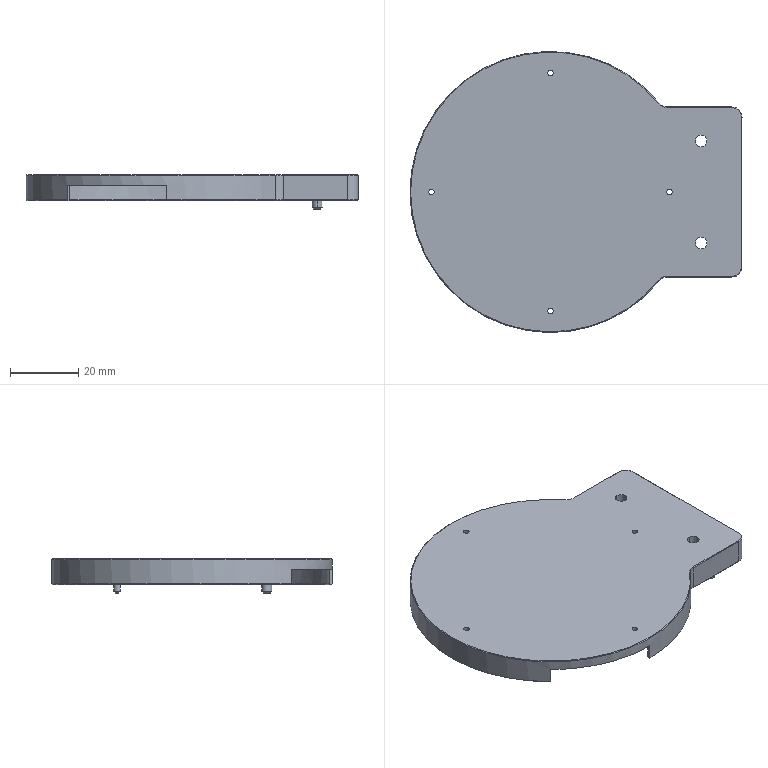NC program | NX | posted with a generic post | part box 97.6 x 82.6 x 10 mm
Lines 2561 to 3495 of 4898:
(CAVITY_MILL_COPY_COPY , TOOL : D3)
N5108 T17 M6
N5110 G54
N5112 G17 G0 G90 X20.005 Y-45.7 S9500 M3
N5114 G43 Z30. H17
N5116 Z-2.196
N5118 G94 G1 Z-2.696 F1000.
N5120 X20.062 Y-45.8
N5122 G3 X20.928 Y-46.3 R1.
N5124 G1 X21.5 F1100.
N5126 G3 X22.5 Y-45.3 R1.
N5128 G1 Y-44.728
N5130 G3 X22. Y-43.862 R1.
N5132 G1 X21.9 Y-43.805
N5134 Z-2.196
N5136 G0 X20.005 Y-45.7 Z-2.391
N5138 G1 Z-2.891 F1000.
N5140 X20.062 Y-45.8
N5142 G3 X20.928 Y-46.3 R1.
N5144 G1 X21.5 F1100.
N5146 G3 X22.5 Y-45.3 R1.
N5148 G1 Y-44.728
N5150 G3 X22. Y-43.862 R1.
N5152 G1 X21.9 Y-43.805
N5154 Z-2.391
N5156 G0 X20.005 Y-45.7 Z-2.587
N5158 G1 Z-3.087 F1000.
N5160 X20.062 Y-45.8
N5162 G3 X20.928 Y-46.3 R1.
N5164 G1 X21.5 F1100.
N5166 G3 X22.5 Y-45.3 R1.
N5168 G1 Y-44.728
N5170 G3 X22. Y-43.862 R1.
N5172 G1 X21.9 Y-43.805
N5174 Z-2.587
N5176 G0 X20.005 Y-45.7 Z-2.783
N5178 G1 Z-3.283 F1000.
N5180 X20.062 Y-45.8
N5182 G3 X20.928 Y-46.3 R1.
N5184 G1 X21.5 F1100.
N5186 G3 X22.5 Y-45.3 R1.
N5188 G1 Y-44.728
N5190 G3 X22. Y-43.862 R1.
N5192 G1 X21.9 Y-43.805
N5194 Z-2.783
N5196 G0 X20.005 Y-45.7 Z-2.978
N5198 G1 Z-3.478 F1000.
N5200 X20.062 Y-45.8
N5202 G3 X20.928 Y-46.3 R1.
N5204 G1 X21.5 F1100.
N5206 G3 X22.5 Y-45.3 R1.
N5208 G1 Y-44.728
N5210 G3 X22. Y-43.862 R1.
N5212 G1 X21.9 Y-43.805
N5214 Z-2.978
N5216 G0 X20.005 Y-45.7 Z-3.174
N5218 G1 Z-3.674 F1000.
N5220 X20.062 Y-45.8
N5222 G3 X20.928 Y-46.3 R1.
N5224 G1 X21.5 F1100.
N5226 G3 X22.5 Y-45.3 R1.
N5228 G1 Y-44.728
N5230 G3 X22. Y-43.862 R1.
N5232 G1 X21.9 Y-43.805
N5234 Z-3.174
N5236 G0 X20.005 Y-45.7 Z-3.37
N5238 G1 Z-3.87 F1000.
N5240 X20.062 Y-45.8
N5242 G3 X20.928 Y-46.3 R1.
N5244 G1 X21.5 F1100.
N5246 G3 X22.5 Y-45.3 R1.
N5248 G1 Y-44.728
N5250 G3 X22. Y-43.862 R1.
N5252 G1 X21.9 Y-43.805
N5254 Z-3.37
N5256 G0 X20.005 Y-45.7 Z-3.565
N5258 G1 Z-4.065 F1000.
N5260 X20.062 Y-45.8
N5262 G3 X20.928 Y-46.3 R1.
N5264 G1 X21.5 F1100.
N5266 G3 X22.5 Y-45.3 R1.
N5268 G1 Y-44.728
N5270 G3 X22. Y-43.862 R1.
N5272 G1 X21.9 Y-43.805
N5274 Z-3.565
N5276 G0 X20.005 Y-45.7 Z-3.761
N5278 G1 Z-4.261 F1000.
N5280 X20.062 Y-45.8
N5282 G3 X20.928 Y-46.3 R1.
N5284 G1 X21.5 F1100.
N5286 G3 X22.5 Y-45.3 R1.
N5288 G1 Y-44.728
N5290 G3 X22. Y-43.862 R1.
N5292 G1 X21.9 Y-43.805
N5294 Z-3.761
N5296 G0 X20.005 Y-45.7 Z-3.957
N5298 G1 Z-4.457 F1000.
N5300 X20.062 Y-45.8
N5302 G3 X20.928 Y-46.3 R1.
N5304 G1 X21.5 F1100.
N5306 G3 X22.5 Y-45.3 R1.
N5308 G1 Y-44.728
N5310 G3 X22. Y-43.862 R1.
N5312 G1 X21.9 Y-43.805
N5314 Z-3.957
N5316 G0 X20.005 Y-45.7 Z-4.152
N5318 G1 Z-4.652 F1000.
N5320 X20.062 Y-45.8
N5322 G3 X20.928 Y-46.3 R1.
N5324 G1 X21.5 F1100.
N5326 G3 X22.5 Y-45.3 R1.
N5328 G1 Y-44.728
N5330 G3 X22. Y-43.862 R1.
N5332 G1 X21.9 Y-43.805
N5334 Z-4.152
N5336 G0 X20.005 Y-45.7 Z-4.348
N5338 G1 Z-4.848 F1000.
N5340 X20.062 Y-45.8
N5342 G3 X20.928 Y-46.3 R1.
N5344 G1 X21.5 F1100.
N5346 G3 X22.5 Y-45.3 R1.
N5348 G1 Y-44.728
N5350 G3 X22. Y-43.862 R1.
N5352 G1 X21.9 Y-43.805
N5354 Z-4.348
N5356 G0 X20.005 Y-45.7 Z-4.543
N5358 G1 Z-5.043 F1000.
N5360 X20.062 Y-45.8
N5362 G3 X20.928 Y-46.3 R1.
N5364 G1 X21.5 F1100.
N5366 G3 X22.5 Y-45.3 R1.
N5368 G1 Y-44.728
N5370 G3 X22. Y-43.862 R1.
N5372 G1 X21.9 Y-43.805
N5374 Z-4.543
N5376 G0 X20.005 Y-45.7 Z-4.739
N5378 G1 Z-5.239 F1000.
N5380 X20.062 Y-45.8
N5382 G3 X20.928 Y-46.3 R1.
N5384 G1 X21.5 F1100.
N5386 G3 X22.5 Y-45.3 R1.
N5388 G1 Y-44.728
N5390 G3 X22. Y-43.862 R1.
N5392 G1 X21.9 Y-43.805
N5394 Z-4.739
N5396 G0 X20.005 Y-45.7 Z-4.935
N5398 G1 Z-5.435 F1000.
N5400 X20.062 Y-45.8
N5402 G3 X20.928 Y-46.3 R1.
N5404 G1 X21.5 F1100.
N5406 G3 X22.5 Y-45.3 R1.
N5408 G1 Y-44.728
N5410 G3 X22. Y-43.862 R1.
N5412 G1 X21.9 Y-43.805
N5414 Z-4.935
N5416 G0 X20.005 Y-45.7 Z-5.13
N5418 G1 Z-5.63 F1000.
N5420 X20.062 Y-45.8
N5422 G3 X20.928 Y-46.3 R1.
N5424 G1 X21.5 F1100.
N5426 G3 X22.5 Y-45.3 R1.
N5428 G1 Y-44.728
N5430 G3 X22. Y-43.862 R1.
N5432 G1 X21.9 Y-43.805
N5434 Z-5.13
N5436 G0 X20.005 Y-45.7 Z-5.326
N5438 G1 Z-5.826 F1000.
N5440 X20.062 Y-45.8
N5442 G3 X20.928 Y-46.3 R1.
N5444 G1 X21.5 F1100.
N5446 G3 X22.5 Y-45.3 R1.
N5448 G1 Y-44.728
N5450 G3 X22. Y-43.862 R1.
N5452 G1 X21.9 Y-43.805
N5454 Z-5.326
N5456 G0 X20.005 Y-45.7 Z-5.522
N5458 G1 Z-6.022 F1000.
N5460 X20.062 Y-45.8
N5462 G3 X20.928 Y-46.3 R1.
N5464 G1 X21.5 F1100.
N5466 G3 X22.5 Y-45.3 R1.
N5468 G1 Y-44.728
N5470 G3 X22. Y-43.862 R1.
N5472 G1 X21.9 Y-43.805
N5474 Z-5.522
N5476 G0 X20.005 Y-45.7 Z-5.717
N5478 G1 Z-6.217 F1000.
N5480 X20.062 Y-45.8
N5482 G3 X20.928 Y-46.3 R1.
N5484 G1 X21.5 F1100.
N5486 G3 X22.5 Y-45.3 R1.
N5488 G1 Y-44.728
N5490 G3 X22. Y-43.862 R1.
N5492 G1 X21.9 Y-43.805
N5494 Z-5.717
N5496 G0 X20.005 Y-45.7 Z-5.913
N5498 G1 Z-6.413 F1000.
N5500 X20.062 Y-45.8
N5502 G3 X20.928 Y-46.3 R1.
N5504 G1 X21.5 F1100.
N5506 G3 X22.5 Y-45.3 R1.
N5508 G1 Y-44.728
N5510 G3 X22. Y-43.862 R1.
N5512 G1 X21.9 Y-43.805
N5514 Z-5.913
N5516 G0 X20.005 Y-45.7 Z-6.109
N5518 G1 Z-6.609 F1000.
N5520 X20.062 Y-45.8
N5522 G3 X20.928 Y-46.3 R1.
N5524 G1 X21.5 F1100.
N5526 G3 X22.5 Y-45.3 R1.
N5528 G1 Y-44.728
N5530 G3 X22. Y-43.862 R1.
N5532 G1 X21.9 Y-43.805
N5534 Z-6.109
N5536 G0 X20.005 Y-45.7 Z-6.304
N5538 G1 Z-6.804 F1000.
N5540 X20.062 Y-45.8
N5542 G3 X20.928 Y-46.3 R1.
N5544 G1 X21.5 F1100.
N5546 G3 X22.5 Y-45.3 R1.
N5548 G1 Y-44.728
N5550 G3 X22. Y-43.862 R1.
N5552 G1 X21.9 Y-43.805
N5554 Z-6.304
N5556 G0 X20.005 Y-45.7 Z-6.5
N5558 G1 Z-7. F1000.
N5560 X20.062 Y-45.8
N5562 G3 X20.928 Y-46.3 R1.
N5564 G1 X21.5 F1100.
N5566 G3 X22.5 Y-45.3 R1.
N5568 G1 Y-44.728
N5570 G3 X22. Y-43.862 R1.
N5572 G1 X21.9 Y-43.805
N5574 Z-6.5
N5576 G0 X20.005 Y-45.7 Z-6.7
N5578 G1 Z-7.2 F1000.
N5580 X20.062 Y-45.8
N5582 G3 X20.928 Y-46.3 R1.
N5584 G1 X21.5 F1100.
N5586 G3 X22.5 Y-45.3 R1.
N5588 G1 Y-44.728
N5590 G3 X22. Y-43.862 R1.
N5592 G1 X21.9 Y-43.805
N5594 Z-6.7
N5596 G0 X20.005 Y-45.7 Z-6.9
N5598 G1 Z-7.4 F1000.
N5600 X20.062 Y-45.8
N5602 G3 X20.928 Y-46.3 R1.
N5604 G1 X21.5 F1100.
N5606 G3 X22.5 Y-45.3 R1.
N5608 G1 Y-44.728
N5610 G3 X22. Y-43.862 R1.
N5612 G1 X21.9 Y-43.805
N5614 Z-6.9
N5616 G0 X20.005 Y-45.7 Z-7.1
N5618 G1 Z-7.6 F1000.
N5620 X20.062 Y-45.8
N5622 G3 X20.928 Y-46.3 R1.
N5624 G1 X21.5 F1100.
N5626 G3 X22.5 Y-45.3 R1.
N5628 G1 Y-44.728
N5630 G3 X22. Y-43.862 R1.
N5632 G1 X21.9 Y-43.805
N5634 Z-7.1
N5636 G0 X20.005 Y-45.7 Z-7.3
N5638 G1 Z-7.8 F1000.
N5640 X20.062 Y-45.8
N5642 G3 X20.928 Y-46.3 R1.
N5644 G1 X21.5 F1100.
N5646 G3 X22.5 Y-45.3 R1.
N5648 G1 Y-44.728
N5650 G3 X22. Y-43.862 R1.
N5652 G1 X21.9 Y-43.805
N5654 Z-7.3
N5656 G0 X20.005 Y-45.7 Z-7.5
N5658 G1 Z-8. F1000.
N5660 X20.062 Y-45.8
N5662 G3 X20.928 Y-46.3 R1.
N5664 G1 X21.5 F1100.
N5666 G3 X22.5 Y-45.3 R1.
N5668 G1 Y-44.728
N5670 G3 X22. Y-43.862 R1.
N5672 G1 X21.9 Y-43.805
N5674 Z-7.5
N5676 G0 X20.005 Y-45.7 Z-7.7
N5678 G1 Z-8.2 F1000.
N5680 X20.062 Y-45.8
N5682 G3 X20.928 Y-46.3 R1.
N5684 G1 X21.5 F1100.
N5686 G3 X22.5 Y-45.3 R1.
N5688 G1 Y-44.728
N5690 G3 X22. Y-43.862 R1.
N5692 G1 X21.9 Y-43.805
N5694 Z-7.7
N5696 G0 X20.005 Y-45.7 Z-7.9
N5698 G1 Z-8.4 F1000.
N5700 X20.062 Y-45.8
N5702 G3 X20.928 Y-46.3 R1.
N5704 G1 X21.5 F1100.
N5706 G3 X22.5 Y-45.3 R1.
N5708 G1 Y-44.728
N5710 G3 X22. Y-43.862 R1.
N5712 G1 X21.9 Y-43.805
N5714 Z-7.9
N5716 G0 X20.005 Y-45.7 Z-8.1
N5718 G1 Z-8.6 F1000.
N5720 X20.062 Y-45.8
N5722 G3 X20.928 Y-46.3 R1.
N5724 G1 X21.5 F1100.
N5726 G3 X22.5 Y-45.3 R1.
N5728 G1 Y-44.728
N5730 G3 X22. Y-43.862 R1.
N5732 G1 X21.9 Y-43.805
N5734 Z-8.1
N5736 G0 X20.005 Y-45.7 Z-8.3
N5738 G1 Z-8.8 F1000.
N5740 X20.062 Y-45.8
N5742 G3 X20.928 Y-46.3 R1.
N5744 G1 X21.5 F1100.
N5746 G3 X22.5 Y-45.3 R1.
N5748 G1 Y-44.728
N5750 G3 X22. Y-43.862 R1.
N5752 G1 X21.9 Y-43.805
N5754 Z-8.3
N5756 G0 X20.005 Y-45.7 Z-8.5
N5758 G1 Z-9. F1000.
N5760 X20.062 Y-45.8
N5762 G3 X20.928 Y-46.3 R1.
N5764 G1 X21.5 F1100.
N5766 G3 X22.5 Y-45.3 R1.
N5768 G1 Y-44.728
N5770 G3 X22. Y-43.862 R1.
N5772 G1 X21.9 Y-43.805
N5774 Z-8.5
N5776 G0 Z30.
N5778 X19.836 Y-31.6
N5780 Z0.5
N5782 G1 X22.176 Z0.377 F1000.
N5784 X22.5 Y-31.276 Z0.353
N5786 Y-29.619 Z0.266
N5788 X22.211 Y-29.309 Z0.244
N5790 X21.88 Y-29.285 Z0.227
N5792 X20.365 Y-30.178 Z0.135
N5794 X18.872 Y-30.948 Z0.047
N5796 X17.408 Y-31.6 Z-0.037
N5798 X22.176 Z-0.287
N5800 X22.5 Y-31.276 Z-0.311
N5802 Y-29.619 Z-0.398
N5804 X22.211 Y-29.309 Z-0.42
N5806 X21.88 Y-29.285 Z-0.438
N5808 X20.365 Y-30.178 Z-0.53
N5810 X18.872 Y-30.948 Z-0.618
N5812 X17.408 Y-31.6 Z-0.702
N5814 X22.176 Z-0.952
N5816 X22.5 Y-31.276 Z-0.976
N5818 Y-29.619 Z-1.063
N5820 X22.211 Y-29.309 Z-1.085
N5822 X21.88 Y-29.285 Z-1.102
N5824 X20.365 Y-30.178 Z-1.194
N5826 X18.872 Y-30.948 Z-1.282
N5828 X17.408 Y-31.6 Z-1.366
N5830 X22.176 Z-1.616
N5832 X22.5 Y-31.276 Z-1.64
N5834 Y-29.619 Z-1.727
N5836 X22.211 Y-29.309 Z-1.749
N5838 X21.88 Y-29.285 Z-1.767
N5840 X20.365 Y-30.178 Z-1.859
N5842 X18.872 Y-30.948 Z-1.947
N5844 X17.408 Y-31.6 Z-2.031
N5846 X22.176 Z-2.281
N5848 X22.5 Y-31.276 Z-2.305
N5850 Y-29.619 Z-2.392
N5852 X22.211 Y-29.309 Z-2.414
N5854 X21.88 Y-29.285 Z-2.431
N5856 X20.365 Y-30.178 Z-2.524
N5858 X18.872 Y-30.948 Z-2.612
N5860 X17.408 Y-31.6 Z-2.696
N5862 X22. F1100.
N5864 G3 X22.5 Y-31.1 R0.5
N5866 G1 Y-29.795
N5868 G3 X21.746 Y-29.364 R0.5
N5870 G2 X17.408 Y-31.6 R42.8
N5872 G3 X17.658 Y-31.533 R0.5
N5874 G1 Z-2.196
N5876 G0 X17.949 Y-31.359
N5878 G1 X17.408 Y-31.6 Z-2.227 F1000.
N5880 X22.176 Z-2.477
N5882 X22.5 Y-31.276 Z-2.501
N5884 Y-29.619 Z-2.587
N5886 X22.211 Y-29.309 Z-2.61
N5888 X21.88 Y-29.285 Z-2.627
N5890 X20.365 Y-30.178 Z-2.719
N5892 X18.872 Y-30.948 Z-2.807
N5894 X17.408 Y-31.6 Z-2.891
N5896 X22. F1100.
N5898 G3 X22.5 Y-31.1 R0.5
N5900 G1 Y-29.795
N5902 G3 X21.746 Y-29.364 R0.5
N5904 G2 X17.408 Y-31.6 R42.8
N5906 G3 X17.658 Y-31.533 R0.5
N5908 G1 Z-2.391
N5910 G0 X17.949 Y-31.359
N5912 G1 X17.408 Y-31.6 Z-2.422 F1000.
N5914 X22.176 Z-2.672
N5916 X22.5 Y-31.276 Z-2.696
N5918 Y-29.619 Z-2.783
N5920 X22.211 Y-29.309 Z-2.805
N5922 X21.88 Y-29.285 Z-2.823
N5924 X20.365 Y-30.178 Z-2.915
N5926 X18.872 Y-30.948 Z-3.003
N5928 X17.408 Y-31.6 Z-3.087
N5930 X22. F1100.
N5932 G3 X22.5 Y-31.1 R0.5
N5934 G1 Y-29.795
N5936 G3 X21.746 Y-29.364 R0.5
N5938 G2 X17.408 Y-31.6 R42.8
N5940 G3 X17.658 Y-31.533 R0.5
N5942 G1 Z-2.587
N5944 G0 X17.949 Y-31.359
N5946 G1 X17.408 Y-31.6 Z-2.618 F1000.
N5948 X22.176 Z-2.868
N5950 X22.5 Y-31.276 Z-2.892
N5952 Y-29.619 Z-2.979
N5954 X22.211 Y-29.309 Z-3.001
N5956 X21.88 Y-29.285 Z-3.018
N5958 X20.365 Y-30.178 Z-3.111
N5960 X18.872 Y-30.948 Z-3.199
N5962 X17.408 Y-31.6 Z-3.283
N5964 X22. F1100.
N5966 G3 X22.5 Y-31.1 R0.5
N5968 G1 Y-29.795
N5970 G3 X21.746 Y-29.364 R0.5
N5972 G2 X17.408 Y-31.6 R42.8
N5974 G3 X17.658 Y-31.533 R0.5
N5976 G1 Z-2.783
N5978 G0 X17.949 Y-31.359
N5980 G1 X17.408 Y-31.6 Z-2.814 F1000.
N5982 X22.176 Z-3.064
N5984 X22.5 Y-31.276 Z-3.088
N5986 Y-29.619 Z-3.174
N5988 X22.211 Y-29.309 Z-3.197
N5990 X21.88 Y-29.285 Z-3.214
N5992 X20.365 Y-30.178 Z-3.306
N5994 X18.872 Y-30.948 Z-3.394
N5996 X17.408 Y-31.6 Z-3.478
N5998 X22. F1100.
N6000 G3 X22.5 Y-31.1 R0.5
N6002 G1 Y-29.795
N6004 G3 X21.746 Y-29.364 R0.5
N6006 G2 X17.408 Y-31.6 R42.8
N6008 G3 X17.658 Y-31.533 R0.5
N6010 G1 Z-2.978
N6012 G0 X17.949 Y-31.359
N6014 G1 X17.408 Y-31.6 Z-3.009 F1000.
N6016 X22.176 Z-3.259
N6018 X22.5 Y-31.276 Z-3.283
N6020 Y-29.619 Z-3.37
N6022 X22.211 Y-29.309 Z-3.392
N6024 X21.88 Y-29.285 Z-3.41
N6026 X20.365 Y-30.178 Z-3.502
N6028 X18.872 Y-30.948 Z-3.59
N6030 X17.408 Y-31.6 Z-3.674
N6032 X22. F1100.
N6034 G3 X22.5 Y-31.1 R0.5
N6036 G1 Y-29.795
N6038 G3 X21.746 Y-29.364 R0.5
N6040 G2 X17.408 Y-31.6 R42.8
N6042 G3 X17.658 Y-31.533 R0.5
N6044 G1 Z-3.174
N6046 G0 X17.949 Y-31.359
N6048 G1 X17.408 Y-31.6 Z-3.205 F1000.
N6050 X22.176 Z-3.455
N6052 X22.5 Y-31.276 Z-3.479
N6054 Y-29.619 Z-3.566
N6056 X22.211 Y-29.309 Z-3.588
N6058 X21.88 Y-29.285 Z-3.605
N6060 X20.365 Y-30.178 Z-3.698
N6062 X18.872 Y-30.948 Z-3.786
N6064 X17.408 Y-31.6 Z-3.87
N6066 X22. F1100.
N6068 G3 X22.5 Y-31.1 R0.5
N6070 G1 Y-29.795
N6072 G3 X21.746 Y-29.364 R0.5
N6074 G2 X17.408 Y-31.6 R42.8
N6076 G3 X17.658 Y-31.533 R0.5
N6078 G1 Z-3.37
N6080 G0 X17.949 Y-31.359
N6082 G1 X17.408 Y-31.6 Z-3.401 F1000.
N6084 X22.176 Z-3.651
N6086 X22.5 Y-31.276 Z-3.675
N6088 Y-29.619 Z-3.761
N6090 X22.211 Y-29.309 Z-3.784
N6092 X21.88 Y-29.285 Z-3.801
N6094 X20.365 Y-30.178 Z-3.893
N6096 X18.872 Y-30.948 Z-3.981
N6098 X17.408 Y-31.6 Z-4.065
N6100 X22. F1100.
N6102 G3 X22.5 Y-31.1 R0.5
N6104 G1 Y-29.795
N6106 G3 X21.746 Y-29.364 R0.5
N6108 G2 X17.408 Y-31.6 R42.8
N6110 G3 X17.658 Y-31.533 R0.5
N6112 G1 Z-3.565
N6114 G0 X17.949 Y-31.359
N6116 G1 X17.408 Y-31.6 Z-3.596 F1000.
N6118 X22.176 Z-3.846
N6120 X22.5 Y-31.276 Z-3.87
N6122 Y-29.619 Z-3.957
N6124 X22.211 Y-29.309 Z-3.979
N6126 X21.88 Y-29.285 Z-3.997
N6128 X20.365 Y-30.178 Z-4.089
N6130 X18.872 Y-30.948 Z-4.177
N6132 X17.408 Y-31.6 Z-4.261
N6134 X22. F1100.
N6136 G3 X22.5 Y-31.1 R0.5
N6138 G1 Y-29.795
N6140 G3 X21.746 Y-29.364 R0.5
N6142 G2 X17.408 Y-31.6 R42.8
N6144 G3 X17.658 Y-31.533 R0.5
N6146 G1 Z-3.761
N6148 G0 X17.949 Y-31.359
N6150 G1 X17.408 Y-31.6 Z-3.792 F1000.
N6152 X22.176 Z-4.042
N6154 X22.5 Y-31.276 Z-4.066
N6156 Y-29.619 Z-4.153
N6158 X22.211 Y-29.309 Z-4.175
N6160 X21.88 Y-29.285 Z-4.192
N6162 X20.365 Y-30.178 Z-4.284
N6164 X18.872 Y-30.948 Z-4.373
N6166 X17.408 Y-31.6 Z-4.457
N6168 X22. F1100.
N6170 G3 X22.5 Y-31.1 R0.5
N6172 G1 Y-29.795
N6174 G3 X21.746 Y-29.364 R0.5
N6176 G2 X17.408 Y-31.6 R42.8
N6178 G3 X17.658 Y-31.533 R0.5
N6180 G1 Z-3.957
N6182 G0 X17.949 Y-31.359
N6184 G1 X17.408 Y-31.6 Z-3.988 F1000.
N6186 X22.176 Z-4.237
N6188 X22.5 Y-31.276 Z-4.262
N6190 Y-29.619 Z-4.348
N6192 X22.211 Y-29.309 Z-4.371
N6194 X21.88 Y-29.285 Z-4.388
N6196 X20.365 Y-30.178 Z-4.48
N6198 X18.872 Y-30.948 Z-4.568
N6200 X17.408 Y-31.6 Z-4.652
N6202 X22. F1100.
N6204 G3 X22.5 Y-31.1 R0.5
N6206 G1 Y-29.795
N6208 G3 X21.746 Y-29.364 R0.5
N6210 G2 X17.408 Y-31.6 R42.8
N6212 G3 X17.658 Y-31.533 R0.5
N6214 G1 Z-4.152
N6216 G0 X17.949 Y-31.359
N6218 G1 X17.408 Y-31.6 Z-4.183 F1000.
N6220 X22.176 Z-4.433
N6222 X22.5 Y-31.276 Z-4.457
N6224 Y-29.619 Z-4.544
N6226 X22.211 Y-29.309 Z-4.566
N6228 X21.88 Y-29.285 Z-4.584
N6230 X20.365 Y-30.178 Z-4.676
N6232 X18.872 Y-30.948 Z-4.764
N6234 X17.408 Y-31.6 Z-4.848
N6236 X22. F1100.
N6238 G3 X22.5 Y-31.1 R0.5
N6240 G1 Y-29.795
N6242 G3 X21.746 Y-29.364 R0.5
N6244 G2 X17.408 Y-31.6 R42.8
N6246 G3 X17.658 Y-31.533 R0.5
N6248 G1 Z-4.348
N6250 G0 X17.949 Y-31.359
N6252 G1 X17.408 Y-31.6 Z-4.379 F1000.
N6254 X22.176 Z-4.629
N6256 X22.5 Y-31.276 Z-4.653
N6258 Y-29.619 Z-4.74
N6260 X22.211 Y-29.309 Z-4.762
N6262 X21.88 Y-29.285 Z-4.779
N6264 X20.365 Y-30.178 Z-4.871
N6266 X18.872 Y-30.948 Z-4.959
N6268 X17.408 Y-31.6 Z-5.043
N6270 X22. F1100.
N6272 G3 X22.5 Y-31.1 R0.5
N6274 G1 Y-29.795
N6276 G3 X21.746 Y-29.364 R0.5
N6278 G2 X17.408 Y-31.6 R42.8
N6280 G3 X17.658 Y-31.533 R0.5
N6282 G1 Z-4.543
N6284 G0 X17.949 Y-31.359
N6286 G1 X17.408 Y-31.6 Z-4.575 F1000.
N6288 X22.176 Z-4.824
N6290 X22.5 Y-31.276 Z-4.848
N6292 Y-29.619 Z-4.935
N6294 X22.211 Y-29.309 Z-4.958
N6296 X21.88 Y-29.285 Z-4.975
N6298 X20.365 Y-30.178 Z-5.067
N6300 X18.872 Y-30.948 Z-5.155
N6302 X17.408 Y-31.6 Z-5.239
N6304 X22. F1100.
N6306 G3 X22.5 Y-31.1 R0.5
N6308 G1 Y-29.795
N6310 G3 X21.746 Y-29.364 R0.5
N6312 G2 X17.408 Y-31.6 R42.8
N6314 G3 X17.658 Y-31.533 R0.5
N6316 G1 Z-4.739
N6318 G0 X17.949 Y-31.359
N6320 G1 X17.408 Y-31.6 Z-4.77 F1000.
N6322 X22.176 Z-5.02
N6324 X22.5 Y-31.276 Z-5.044
N6326 Y-29.619 Z-5.131
N6328 X22.211 Y-29.309 Z-5.153
N6330 X21.88 Y-29.285 Z-5.171
N6332 X20.365 Y-30.178 Z-5.263
N6334 X18.872 Y-30.948 Z-5.351
N6336 X17.408 Y-31.6 Z-5.435
N6338 X22. F1100.
N6340 G3 X22.5 Y-31.1 R0.5
N6342 G1 Y-29.795
N6344 G3 X21.746 Y-29.364 R0.5
N6346 G2 X17.408 Y-31.6 R42.8
N6348 G3 X17.658 Y-31.533 R0.5
N6350 G1 Z-4.935
N6352 G0 X17.949 Y-31.359
N6354 G1 X17.408 Y-31.6 Z-4.966 F1000.
N6356 X22.176 Z-5.216
N6358 X22.5 Y-31.276 Z-5.24
N6360 Y-29.619 Z-5.327
N6362 X22.211 Y-29.309 Z-5.349
N6364 X21.88 Y-29.285 Z-5.366
N6366 X20.365 Y-30.178 Z-5.458
N6368 X18.872 Y-30.948 Z-5.546
N6370 X17.408 Y-31.6 Z-5.63
N6372 X22. F1100.
N6374 G3 X22.5 Y-31.1 R0.5
N6376 G1 Y-29.795
N6378 G3 X21.746 Y-29.364 R0.5
N6380 G2 X17.408 Y-31.6 R42.8
N6382 G3 X17.658 Y-31.533 R0.5
N6384 G1 Z-5.13
N6386 G0 X17.949 Y-31.359
N6388 G1 X17.408 Y-31.6 Z-5.162 F1000.
N6390 X22.176 Z-5.411
N6392 X22.5 Y-31.276 Z-5.435
N6394 Y-29.619 Z-5.522
N6396 X22.211 Y-29.309 Z-5.544
N6398 X21.88 Y-29.285 Z-5.562
N6400 X20.365 Y-30.178 Z-5.654
N6402 X18.872 Y-30.948 Z-5.742
N6404 X17.408 Y-31.6 Z-5.826
N6406 X22. F1100.
N6408 G3 X22.5 Y-31.1 R0.5
N6410 G1 Y-29.795
N6412 G3 X21.746 Y-29.364 R0.5
N6414 G2 X17.408 Y-31.6 R42.8
N6416 G3 X17.658 Y-31.533 R0.5
N6418 G1 Z-5.326
N6420 G0 X17.949 Y-31.359
N6422 G1 X17.408 Y-31.6 Z-5.357 F1000.
N6424 X22.176 Z-5.607
N6426 X22.5 Y-31.276 Z-5.631
N6428 Y-29.619 Z-5.718
N6430 X22.211 Y-29.309 Z-5.74
N6432 X21.88 Y-29.285 Z-5.758
N6434 X20.365 Y-30.178 Z-5.85
N6436 X18.872 Y-30.948 Z-5.938
N6438 X17.408 Y-31.6 Z-6.022
N6440 X22. F1100.
N6442 G3 X22.5 Y-31.1 R0.5
N6444 G1 Y-29.795
N6446 G3 X21.746 Y-29.364 R0.5
N6448 G2 X17.408 Y-31.6 R42.8
N6450 G3 X17.658 Y-31.533 R0.5
N6452 G1 Z-5.522
N6454 G0 X17.949 Y-31.359
N6456 G1 X17.408 Y-31.6 Z-5.553 F1000.
N6458 X22.176 Z-5.803
N6460 X22.5 Y-31.276 Z-5.827
N6462 Y-29.619 Z-5.914
N6464 X22.211 Y-29.309 Z-5.936
N6466 X21.88 Y-29.285 Z-5.953
N6468 X20.365 Y-30.178 Z-6.045
N6470 X18.872 Y-30.948 Z-6.133
N6472 X17.408 Y-31.6 Z-6.217
N6474 X22. F1100.
N6476 G3 X22.5 Y-31.1 R0.5
N6478 G1 Y-29.795
N6480 G3 X21.746 Y-29.364 R0.5
N6482 G2 X17.408 Y-31.6 R42.8
N6484 G3 X17.658 Y-31.533 R0.5
N6486 G1 Z-5.717
N6488 G0 X17.949 Y-31.359
N6490 G1 X17.408 Y-31.6 Z-5.748 F1000.
N6492 X22.176 Z-5.998
N6494 X22.5 Y-31.276 Z-6.022
N6496 Y-29.619 Z-6.109
N6498 X22.211 Y-29.309 Z-6.131
N6500 X21.88 Y-29.285 Z-6.149
N6502 X20.365 Y-30.178 Z-6.241
N6504 X18.872 Y-30.948 Z-6.329
N6506 X17.408 Y-31.6 Z-6.413
N6508 X22. F1100.
N6510 G3 X22.5 Y-31.1 R0.5
N6512 G1 Y-29.795
N6514 G3 X21.746 Y-29.364 R0.5
N6516 G2 X17.408 Y-31.6 R42.8
N6518 G3 X17.658 Y-31.533 R0.5
N6520 G1 Z-5.913
N6522 G0 X17.949 Y-31.359
N6524 G1 X17.408 Y-31.6 Z-5.944 F1000.
N6526 X22.176 Z-6.194
N6528 X22.5 Y-31.276 Z-6.218
N6530 Y-29.619 Z-6.305
N6532 X22.211 Y-29.309 Z-6.327
N6534 X21.88 Y-29.285 Z-6.344
N6536 X20.365 Y-30.178 Z-6.437
N6538 X18.872 Y-30.948 Z-6.525
N6540 X17.408 Y-31.6 Z-6.609
N6542 X22. F1100.
N6544 G3 X22.5 Y-31.1 R0.5
N6546 G1 Y-29.795
N6548 G3 X21.746 Y-29.364 R0.5
N6550 G2 X17.408 Y-31.6 R42.8
N6552 G3 X17.658 Y-31.533 R0.5
N6554 G1 Z-6.109
N6556 G0 X17.949 Y-31.359
N6558 G1 X17.408 Y-31.6 Z-6.14 F1000.
N6560 X22.176 Z-6.39
N6562 X22.5 Y-31.276 Z-6.414
N6564 Y-29.619 Z-6.501
N6566 X22.211 Y-29.309 Z-6.523
N6568 X21.88 Y-29.285 Z-6.54
N6570 X20.365 Y-30.178 Z-6.632
N6572 X18.872 Y-30.948 Z-6.72
N6574 X17.408 Y-31.6 Z-6.804
N6576 X22. F1100.
N6578 G3 X22.5 Y-31.1 R0.5
N6580 G1 Y-29.795
N6582 G3 X21.746 Y-29.364 R0.5
N6584 G2 X17.408 Y-31.6 R42.8
N6586 G3 X17.658 Y-31.533 R0.5
N6588 G1 Z-6.304
N6590 G0 X17.949 Y-31.359
N6592 G1 X17.408 Y-31.6 Z-6.335 F1000.
N6594 X22.176 Z-6.585
N6596 X22.5 Y-31.276 Z-6.609
N6598 Y-29.619 Z-6.696
N6600 X22.211 Y-29.309 Z-6.718
N6602 X21.88 Y-29.285 Z-6.736
N6604 X20.365 Y-30.178 Z-6.828
N6606 X18.872 Y-30.948 Z-6.916
N6608 X17.408 Y-31.6 Z-7.
N6610 X22. F1100.
N6612 G3 X22.5 Y-31.1 R0.5
N6614 G1 Y-29.795
N6616 G3 X21.746 Y-29.364 R0.5
N6618 G2 X17.408 Y-31.6 R42.8
N6620 G3 X17.658 Y-31.533 R0.5
N6622 G1 Z-6.5
N6624 G0 X18.025 Y-31.325
N6626 G1 X17.408 Y-31.6 Z-6.535 F1000.
N6628 X22.176 Z-6.785
N6630 X22.5 Y-31.276 Z-6.809
N6632 Y-29.619 Z-6.896
N6634 X22.211 Y-29.309 Z-6.918
N6636 X21.88 Y-29.285 Z-6.936
N6638 X20.365 Y-30.178 Z-7.028
N6640 X18.872 Y-30.948 Z-7.116
N6642 X17.408 Y-31.6 Z-7.2
N6644 X22. F1100.
N6646 G3 X22.5 Y-31.1 R0.5
N6648 G1 Y-29.795
N6650 G3 X21.746 Y-29.364 R0.5
N6652 G2 X17.408 Y-31.6 R42.8
N6654 G3 X17.658 Y-31.533 R0.5
N6656 G1 Z-6.7
N6658 G0 X18.025 Y-31.325
N6660 G1 X17.408 Y-31.6 Z-6.735 F1000.
N6662 X22.176 Z-6.985
N6664 X22.5 Y-31.276 Z-7.009
N6666 Y-29.619 Z-7.096
N6668 X22.211 Y-29.309 Z-7.118
N6670 X21.88 Y-29.285 Z-7.136
N6672 X20.365 Y-30.178 Z-7.228
N6674 X18.872 Y-30.948 Z-7.316
N6676 X17.408 Y-31.6 Z-7.4
N6678 X22. F1100.
N6680 G3 X22.5 Y-31.1 R0.5
N6682 G1 Y-29.795
N6684 G3 X21.746 Y-29.364 R0.5
N6686 G2 X17.408 Y-31.6 R42.8
N6688 G3 X17.658 Y-31.533 R0.5
N6690 G1 Z-6.9
N6692 G0 X18.025 Y-31.325
N6694 G1 X17.408 Y-31.6 Z-6.935 F1000.
N6696 X22.176 Z-7.185
N6698 X22.5 Y-31.276 Z-7.209
N6700 Y-29.619 Z-7.296
N6702 X22.211 Y-29.309 Z-7.318
N6704 X21.88 Y-29.285 Z-7.336
N6706 X20.365 Y-30.178 Z-7.428
N6708 X18.872 Y-30.948 Z-7.516
N6710 X17.408 Y-31.6 Z-7.6
N6712 X22. F1100.
N6714 G3 X22.5 Y-31.1 R0.5
N6716 G1 Y-29.795
N6718 G3 X21.746 Y-29.364 R0.5
N6720 G2 X17.408 Y-31.6 R42.8
N6722 G3 X17.658 Y-31.533 R0.5
N6724 G1 Z-7.1
N6726 G0 X18.025 Y-31.325
N6728 G1 X17.408 Y-31.6 Z-7.135 F1000.
N6730 X22.176 Z-7.385
N6732 X22.5 Y-31.276 Z-7.409
N6734 Y-29.619 Z-7.496
N6736 X22.211 Y-29.309 Z-7.518
N6738 X21.88 Y-29.285 Z-7.536
N6740 X20.365 Y-30.178 Z-7.628
N6742 X18.872 Y-30.948 Z-7.716
N6744 X17.408 Y-31.6 Z-7.8
N6746 X22. F1100.
N6748 G3 X22.5 Y-31.1 R0.5
N6750 G1 Y-29.795
N6752 G3 X21.746 Y-29.364 R0.5
N6754 G2 X17.408 Y-31.6 R42.8
N6756 G3 X17.658 Y-31.533 R0.5
N6758 G1 Z-7.3
N6760 G0 X18.025 Y-31.325
N6762 G1 X17.408 Y-31.6 Z-7.335 F1000.
N6764 X22.176 Z-7.585
N6766 X22.5 Y-31.276 Z-7.609
N6768 Y-29.619 Z-7.696
N6770 X22.211 Y-29.309 Z-7.718
N6772 X21.88 Y-29.285 Z-7.736
N6774 X20.365 Y-30.178 Z-7.828
N6776 X18.872 Y-30.948 Z-7.916
N6778 X17.408 Y-31.6 Z-8.
N6780 X22. F1100.
N6782 G3 X22.5 Y-31.1 R0.5
N6784 G1 Y-29.795
N6786 G3 X21.746 Y-29.364 R0.5
N6788 G2 X17.408 Y-31.6 R42.8
N6790 G3 X17.658 Y-31.533 R0.5
N6792 G1 Z-7.5
N6794 G0 X18.025 Y-31.325
N6796 G1 X17.408 Y-31.6 Z-7.535 F1000.
N6798 X22.176 Z-7.785
N6800 X22.5 Y-31.276 Z-7.809
N6802 Y-29.619 Z-7.896
N6804 X22.211 Y-29.309 Z-7.918
N6806 X21.88 Y-29.285 Z-7.936
N6808 X20.365 Y-30.178 Z-8.028
N6810 X18.872 Y-30.948 Z-8.116
N6812 X17.408 Y-31.6 Z-8.2
N6814 X22. F1100.
N6816 G3 X22.5 Y-31.1 R0.5
N6818 G1 Y-29.795
N6820 G3 X21.746 Y-29.364 R0.5
N6822 G2 X17.408 Y-31.6 R42.8
N6824 G3 X17.658 Y-31.533 R0.5
N6826 G1 Z-7.7
N6828 G0 X18.025 Y-31.325
N6830 G1 X17.408 Y-31.6 Z-7.735 F1000.
N6832 X22.176 Z-7.985
N6834 X22.5 Y-31.276 Z-8.009
N6836 Y-29.619 Z-8.096
N6838 X22.211 Y-29.309 Z-8.118
N6840 X21.88 Y-29.285 Z-8.136
N6842 X20.365 Y-30.178 Z-8.228
N6844 X18.872 Y-30.948 Z-8.316
N6846 X17.408 Y-31.6 Z-8.4
N6848 X22. F1100.
N6850 G3 X22.5 Y-31.1 R0.5
N6852 G1 Y-29.795
N6854 G3 X21.746 Y-29.364 R0.5
N6856 G2 X17.408 Y-31.6 R42.8
N6858 G3 X17.658 Y-31.533 R0.5
N6860 G1 Z-7.9
N6862 G0 X18.025 Y-31.325
N6864 G1 X17.408 Y-31.6 Z-7.935 F1000.
N6866 X22.176 Z-8.185
N6868 X22.5 Y-31.276 Z-8.209
N6870 Y-29.619 Z-8.296
N6872 X22.211 Y-29.309 Z-8.318
N6874 X21.88 Y-29.285 Z-8.336
N6876 X20.365 Y-30.178 Z-8.428
N6878 X18.872 Y-30.948 Z-8.516
N6880 X17.408 Y-31.6 Z-8.6
N6882 X22. F1100.
N6884 G3 X22.5 Y-31.1 R0.5
N6886 G1 Y-29.795
N6888 G3 X21.746 Y-29.364 R0.5
N6890 G2 X17.408 Y-31.6 R42.8
N6892 G3 X17.658 Y-31.533 R0.5
N6894 G1 Z-8.1
N6896 G0 X18.025 Y-31.325
N6898 G1 X17.408 Y-31.6 Z-8.135 F1000.
N6900 X22.176 Z-8.385
N6902 X22.5 Y-31.276 Z-8.409
N6904 Y-29.619 Z-8.496
N6906 X22.211 Y-29.309 Z-8.518
N6908 X21.88 Y-29.285 Z-8.536
N6910 X20.365 Y-30.178 Z-8.628
N6912 X18.872 Y-30.948 Z-8.716
N6914 X17.408 Y-31.6 Z-8.8
N6916 X22. F1100.
N6918 G3 X22.5 Y-31.1 R0.5
N6920 G1 Y-29.795
N6922 G3 X21.746 Y-29.364 R0.5
N6924 G2 X17.408 Y-31.6 R42.8
N6926 G3 X17.658 Y-31.533 R0.5
N6928 G1 Z-8.3
N6930 G0 X18.025 Y-31.325
N6932 G1 X17.408 Y-31.6 Z-8.335 F1000.
N6934 X22.176 Z-8.585
N6936 X22.5 Y-31.276 Z-8.609
N6938 Y-29.619 Z-8.696
N6940 X22.211 Y-29.309 Z-8.718
N6942 X21.88 Y-29.285 Z-8.736
N6944 X20.365 Y-30.178 Z-8.828
N6946 X18.872 Y-30.948 Z-8.916
N6948 X17.408 Y-31.6 Z-9.
N6950 X22. F1100.
N6952 G3 X22.5 Y-31.1 R0.5
N6954 G1 Y-29.795
N6956 G3 X21.746 Y-29.364 R0.5
N6958 G2 X17.408 Y-31.6 R42.8
N6960 G3 X17.658 Y-31.533 R0.5
N6962 G1 Z-8.5
N6964 G0 Z30.
N6966 X-19.843 Y-31.6
N6968 Z0.5
N6970 G1 X-17.685 Z0.387 F1000.